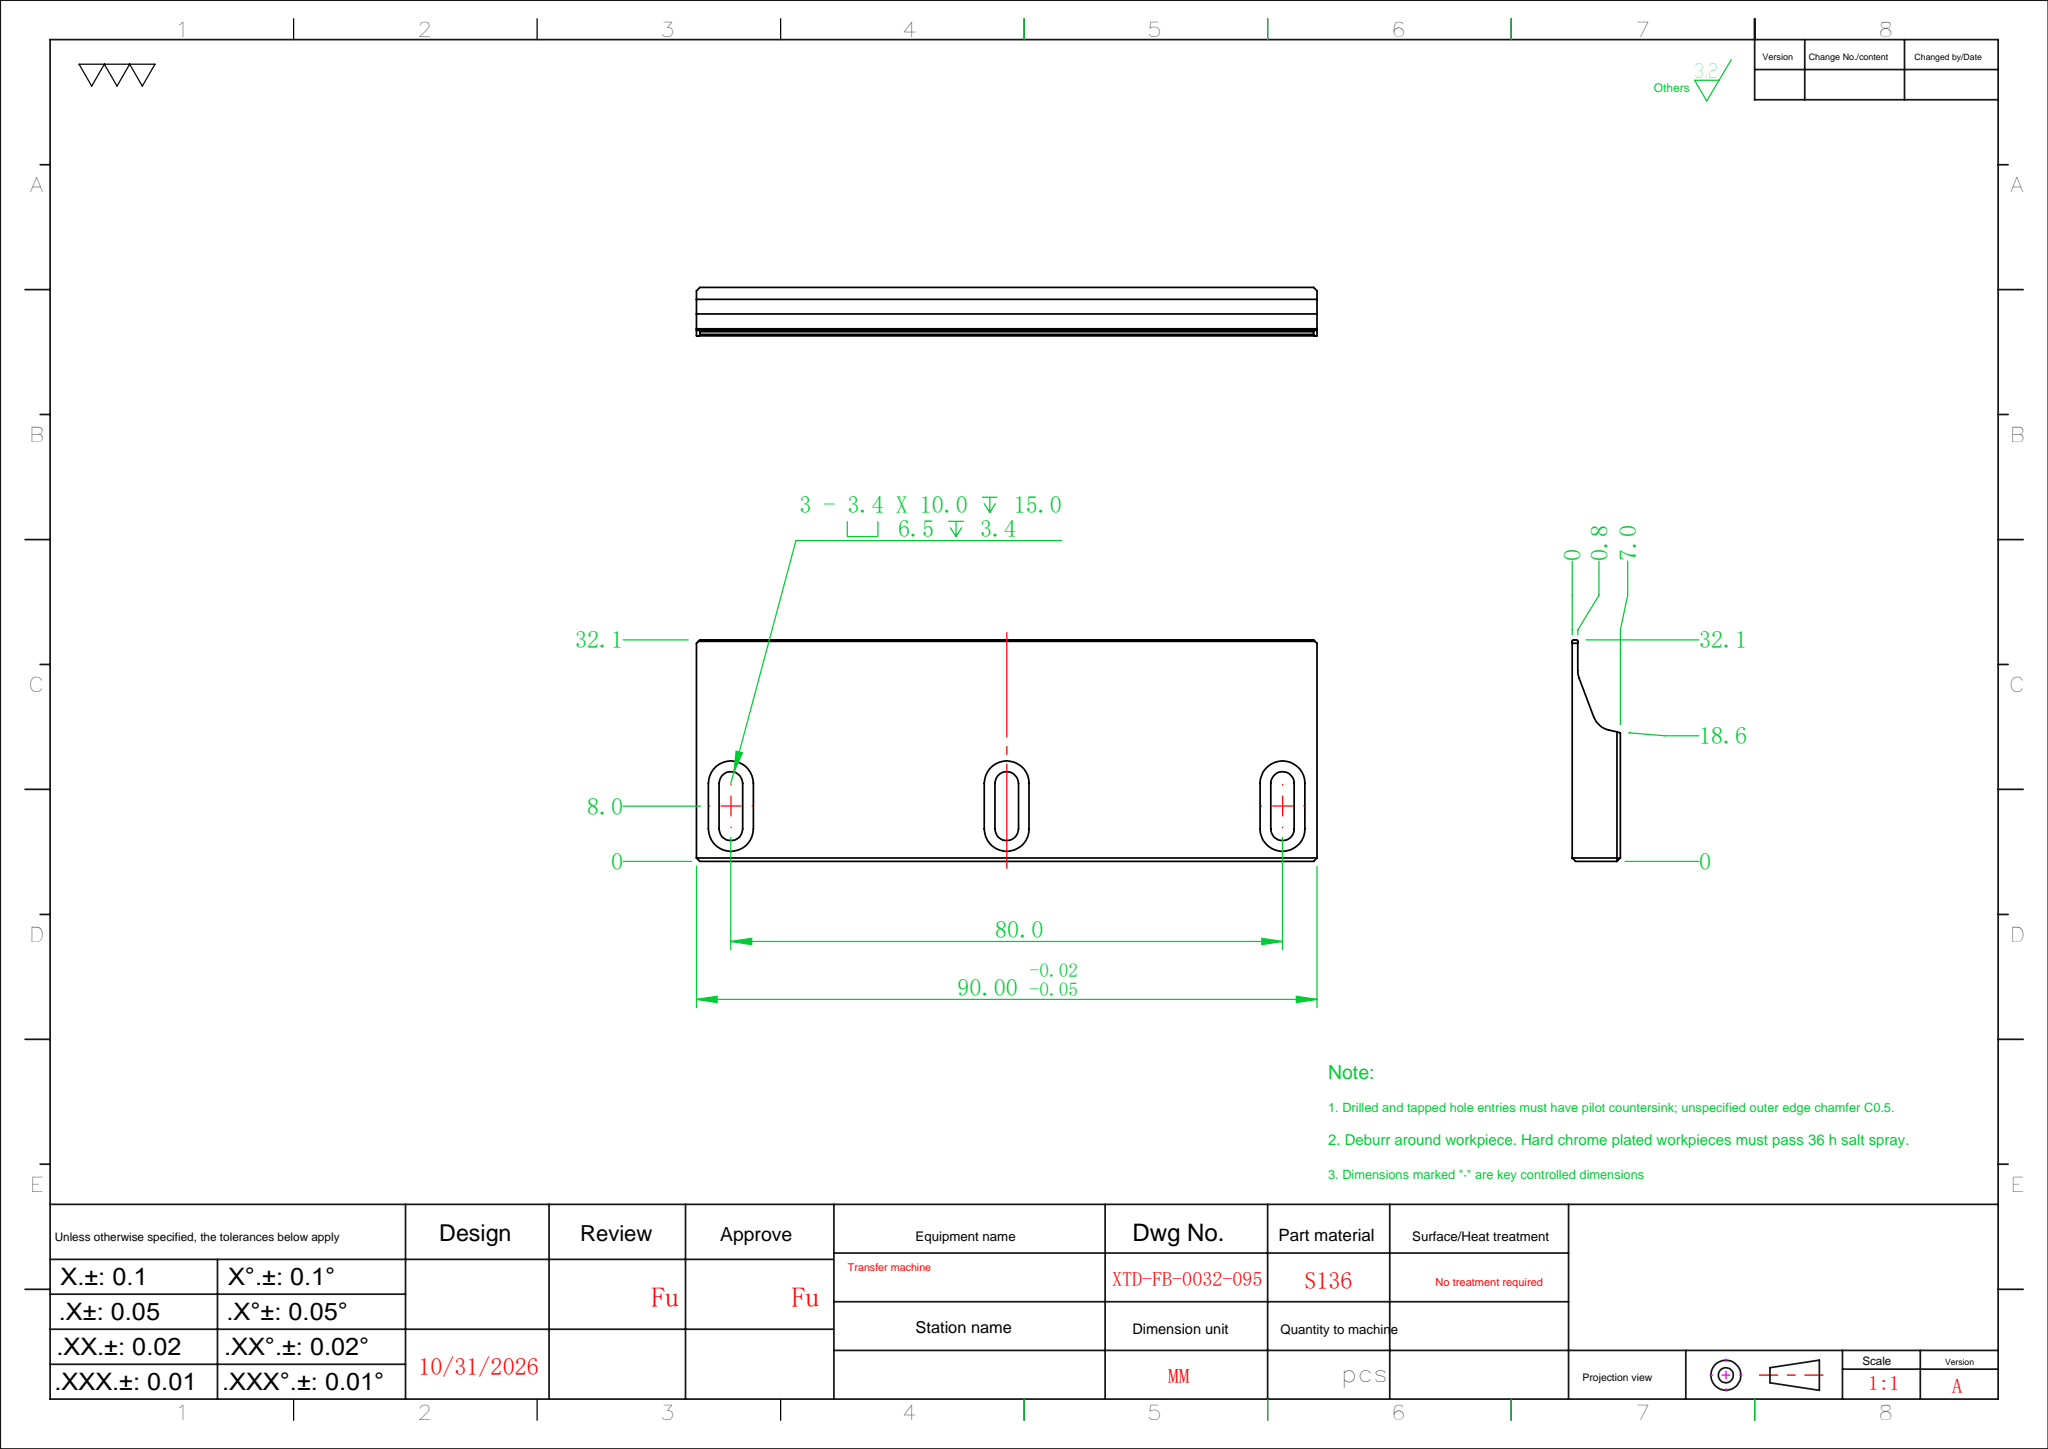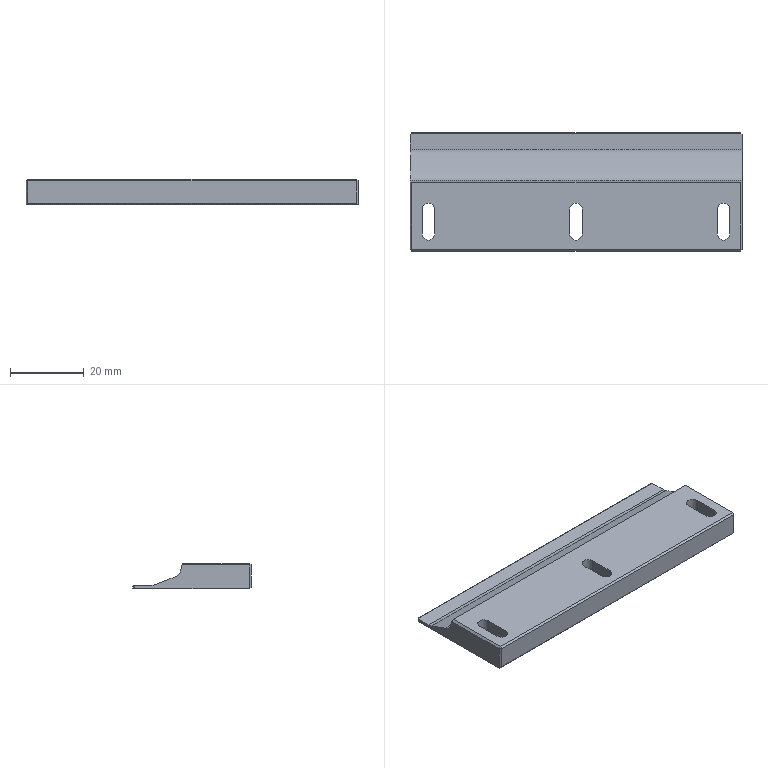Part | SolidWorks | features Chamfer 3, Fillet 2, Extrusion 1, HoleWzd 1, ICE 1 | 1 solid | 50 faces | box 90 x 32.1 x 7 mm | volume 12925 mm3 | plane 34 | cylinder 16 | commonest cylinder face diameters 3.4 x6 6.5 x6 0.4 x2 6 x2